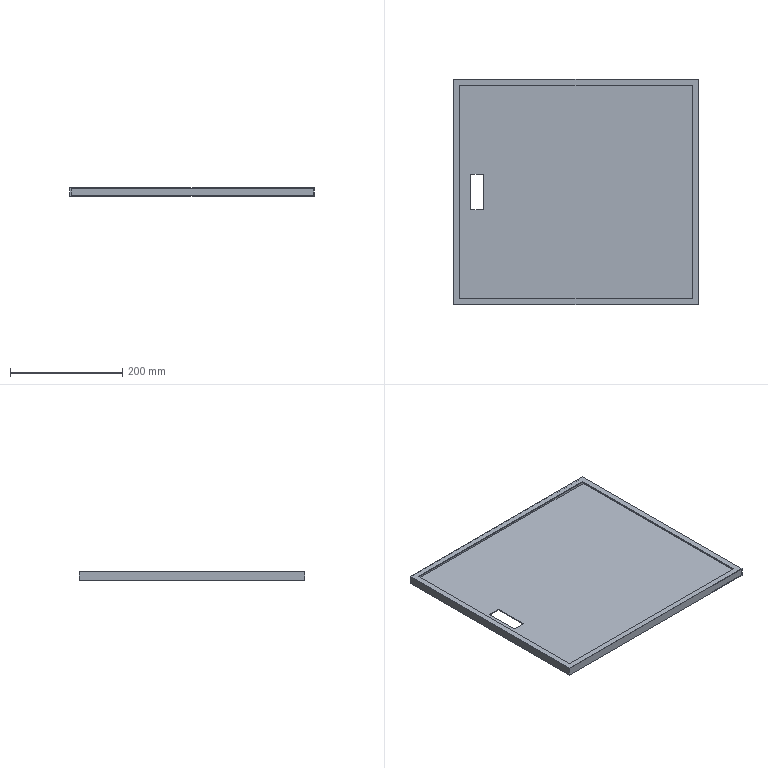Part | 1 solid | 20 faces | box 435.25 x 401 x 15 mm | volume 314971 mm3 | plane 20
STEP:
#1=CARTESIAN_POINT('',(435.25,0.,-625.));
#2=VERTEX_POINT('',#1);
#3=CARTESIAN_POINT('',(435.25,401.,-625.));
#4=VERTEX_POINT('',#3);
#5=CARTESIAN_POINT('',(435.25,0.,-625.));
#6=DIRECTION('',(0.,1.,0.));
#7=VECTOR('',#6,1000.);
#8=LINE('',#5,#7);
#9=EDGE_CURVE('',#2,#4,#8,.T.);
#10=ORIENTED_EDGE('',*,*,#9,.F.);
#11=CARTESIAN_POINT('',(435.25,0.,-640.));
#12=VERTEX_POINT('',#11);
#13=CARTESIAN_POINT('',(435.25,0.,-640.));
#14=DIRECTION('',(0.,0.,1.));
#15=VECTOR('',#14,1000.);
#16=LINE('',#13,#15);
#17=EDGE_CURVE('',#12,#2,#16,.T.);
#18=ORIENTED_EDGE('',*,*,#17,.F.);
#19=CARTESIAN_POINT('',(435.25,401.,-640.));
#20=VERTEX_POINT('',#19);
#21=CARTESIAN_POINT('',(435.25,0.,-640.));
#22=DIRECTION('',(0.,1.,0.));
#23=VECTOR('',#22,1000.);
#24=LINE('',#21,#23);
#25=EDGE_CURVE('',#12,#20,#24,.T.);
#26=ORIENTED_EDGE('',*,*,#25,.T.);
#27=CARTESIAN_POINT('',(435.25,401.,-640.));
#28=DIRECTION('',(0.,0.,1.));
#29=VECTOR('',#28,1000.);
#30=LINE('',#27,#29);
#31=EDGE_CURVE('',#20,#4,#30,.T.);
#32=ORIENTED_EDGE('',*,*,#31,.T.);
#33=EDGE_LOOP('',(#10,#18,#26,#32));
#34=FACE_OUTER_BOUND('',#33,.T.);
#35=CARTESIAN_POINT('',(435.25,0.,-640.));
#36=DIRECTION('',(1.,0.,0.));
#37=DIRECTION('',(0.,1.,0.));
#38=AXIS2_PLACEMENT_3D('',#35,#36,#37);
#39=PLANE('',#38);
#40=ADVANCED_FACE('',(#34),#39,.T.);
#41=CARTESIAN_POINT('',(0.,0.,-625.));
#42=VERTEX_POINT('',#41);
#43=CARTESIAN_POINT('',(0.,0.,-625.));
#44=DIRECTION('',(1.,0.,0.));
#45=VECTOR('',#44,1000.);
#46=LINE('',#43,#45);
#47=EDGE_CURVE('',#42,#2,#46,.T.);
#48=ORIENTED_EDGE('',*,*,#47,.F.);
#49=CARTESIAN_POINT('',(0.,0.,-640.));
#50=VERTEX_POINT('',#49);
#51=CARTESIAN_POINT('',(0.,0.,-640.));
#52=DIRECTION('',(0.,0.,1.));
#53=VECTOR('',#52,1000.);
#54=LINE('',#51,#53);
#55=EDGE_CURVE('',#50,#42,#54,.T.);
#56=ORIENTED_EDGE('',*,*,#55,.F.);
#57=CARTESIAN_POINT('',(0.,0.,-640.));
#58=DIRECTION('',(1.,0.,0.));
#59=VECTOR('',#58,1000.);
#60=LINE('',#57,#59);
#61=EDGE_CURVE('',#50,#12,#60,.T.);
#62=ORIENTED_EDGE('',*,*,#61,.T.);
#63=ORIENTED_EDGE('',*,*,#17,.T.);
#64=EDGE_LOOP('',(#48,#56,#62,#63));
#65=FACE_OUTER_BOUND('',#64,.T.);
#66=CARTESIAN_POINT('',(0.,0.,-640.));
#67=DIRECTION('',(0.,-1.,0.));
#68=DIRECTION('',(0.,0.,-1.));
#69=AXIS2_PLACEMENT_3D('',#66,#67,#68);
#70=PLANE('',#69);
#71=ADVANCED_FACE('',(#65),#70,.T.);
#72=CARTESIAN_POINT('',(0.,401.,-625.));
#73=VERTEX_POINT('',#72);
#74=CARTESIAN_POINT('',(0.,401.,-625.));
#75=DIRECTION('',(0.,-1.,0.));
#76=VECTOR('',#75,1000.);
#77=LINE('',#74,#76);
#78=EDGE_CURVE('',#73,#42,#77,.T.);
#79=ORIENTED_EDGE('',*,*,#78,.F.);
#80=CARTESIAN_POINT('',(0.,401.,-640.));
#81=VERTEX_POINT('',#80);
#82=CARTESIAN_POINT('',(0.,401.,-640.));
#83=DIRECTION('',(0.,0.,1.));
#84=VECTOR('',#83,1000.);
#85=LINE('',#82,#84);
#86=EDGE_CURVE('',#81,#73,#85,.T.);
#87=ORIENTED_EDGE('',*,*,#86,.F.);
#88=CARTESIAN_POINT('',(0.,401.,-640.));
#89=DIRECTION('',(0.,-1.,0.));
#90=VECTOR('',#89,1000.);
#91=LINE('',#88,#90);
#92=EDGE_CURVE('',#81,#50,#91,.T.);
#93=ORIENTED_EDGE('',*,*,#92,.T.);
#94=ORIENTED_EDGE('',*,*,#55,.T.);
#95=EDGE_LOOP('',(#79,#87,#93,#94));
#96=FACE_OUTER_BOUND('',#95,.T.);
#97=CARTESIAN_POINT('',(0.,401.,-640.));
#98=DIRECTION('',(-1.,0.,0.));
#99=DIRECTION('',(0.,-1.,0.));
#100=AXIS2_PLACEMENT_3D('',#97,#98,#99);
#101=PLANE('',#100);
#102=ADVANCED_FACE('',(#96),#101,.T.);
#103=CARTESIAN_POINT('',(435.25,401.,-625.));
#104=DIRECTION('',(-1.,0.,0.));
#105=VECTOR('',#104,1000.);
#106=LINE('',#103,#105);
#107=EDGE_CURVE('',#4,#73,#106,.T.);
#108=ORIENTED_EDGE('',*,*,#107,.F.);
#109=ORIENTED_EDGE('',*,*,#31,.F.);
#110=CARTESIAN_POINT('',(435.25,401.,-640.));
#111=DIRECTION('',(-1.,0.,0.));
#112=VECTOR('',#111,1000.);
#113=LINE('',#110,#112);
#114=EDGE_CURVE('',#20,#81,#113,.T.);
#115=ORIENTED_EDGE('',*,*,#114,.T.);
#116=ORIENTED_EDGE('',*,*,#86,.T.);
#117=EDGE_LOOP('',(#108,#109,#115,#116));
#118=FACE_OUTER_BOUND('',#117,.T.);
#119=CARTESIAN_POINT('',(435.25,401.,-640.));
#120=DIRECTION('',(0.,1.,0.));
#121=DIRECTION('',(0.,0.,1.));
#122=AXIS2_PLACEMENT_3D('',#119,#120,#121);
#123=PLANE('',#122);
#124=ADVANCED_FACE('',(#118),#123,.T.);
#125=CARTESIAN_POINT('',(30.,232.,-640.));
#126=VERTEX_POINT('',#125);
#127=CARTESIAN_POINT('',(53.,232.,-640.));
#128=VERTEX_POINT('',#127);
#129=CARTESIAN_POINT('',(53.,232.,-640.));
#130=DIRECTION('',(1.,0.,0.));
#131=VECTOR('',#130,1000.);
#132=LINE('',#129,#131);
#133=EDGE_CURVE('',#126,#128,#132,.T.);
#134=ORIENTED_EDGE('',*,*,#133,.F.);
#135=CARTESIAN_POINT('',(30.,169.,-640.));
#136=VERTEX_POINT('',#135);
#137=CARTESIAN_POINT('',(30.,232.,-640.));
#138=DIRECTION('',(0.,1.,0.));
#139=VECTOR('',#138,1000.);
#140=LINE('',#137,#139);
#141=EDGE_CURVE('',#136,#126,#140,.T.);
#142=ORIENTED_EDGE('',*,*,#141,.F.);
#143=CARTESIAN_POINT('',(53.,169.,-640.));
#144=VERTEX_POINT('',#143);
#145=CARTESIAN_POINT('',(53.,169.,-640.));
#146=DIRECTION('',(-1.,0.,0.));
#147=VECTOR('',#146,1000.);
#148=LINE('',#145,#147);
#149=EDGE_CURVE('',#144,#136,#148,.T.);
#150=ORIENTED_EDGE('',*,*,#149,.F.);
#151=CARTESIAN_POINT('',(53.,232.,-640.));
#152=DIRECTION('',(0.,-1.,0.));
#153=VECTOR('',#152,1000.);
#154=LINE('',#151,#153);
#155=EDGE_CURVE('',#128,#144,#154,.T.);
#156=ORIENTED_EDGE('',*,*,#155,.F.);
#157=EDGE_LOOP('',(#134,#142,#150,#156));
#158=FACE_BOUND('',#157,.T.);
#159=ORIENTED_EDGE('',*,*,#25,.F.);
#160=ORIENTED_EDGE('',*,*,#61,.F.);
#161=ORIENTED_EDGE('',*,*,#92,.F.);
#162=ORIENTED_EDGE('',*,*,#114,.F.);
#163=EDGE_LOOP('',(#159,#160,#161,#162));
#164=FACE_OUTER_BOUND('',#163,.T.);
#165=CARTESIAN_POINT('',(0.,0.,-640.));
#166=DIRECTION('',(0.,0.,1.));
#167=DIRECTION('',(1.,0.,0.));
#168=AXIS2_PLACEMENT_3D('',#165,#166,#167);
#169=PLANE('',#168);
#170=ADVANCED_FACE('',(#158,#164),#169,.F.);
#171=CARTESIAN_POINT('',(424.5,10.,-625.));
#172=VERTEX_POINT('',#171);
#173=CARTESIAN_POINT('',(10.75,10.,-625.));
#174=VERTEX_POINT('',#173);
#175=CARTESIAN_POINT('',(424.5,10.,-625.));
#176=DIRECTION('',(-1.,0.,0.));
#177=VECTOR('',#176,1000.);
#178=LINE('',#175,#177);
#179=EDGE_CURVE('',#172,#174,#178,.T.);
#180=ORIENTED_EDGE('',*,*,#179,.T.);
#181=CARTESIAN_POINT('',(10.75,391.,-625.));
#182=VERTEX_POINT('',#181);
#183=CARTESIAN_POINT('',(10.75,10.,-625.));
#184=DIRECTION('',(0.,1.,0.));
#185=VECTOR('',#184,1000.);
#186=LINE('',#183,#185);
#187=EDGE_CURVE('',#174,#182,#186,.T.);
#188=ORIENTED_EDGE('',*,*,#187,.T.);
#189=CARTESIAN_POINT('',(424.5,391.,-625.));
#190=VERTEX_POINT('',#189);
#191=CARTESIAN_POINT('',(10.75,391.,-625.));
#192=DIRECTION('',(1.,0.,0.));
#193=VECTOR('',#192,1000.);
#194=LINE('',#191,#193);
#195=EDGE_CURVE('',#182,#190,#194,.T.);
#196=ORIENTED_EDGE('',*,*,#195,.T.);
#197=CARTESIAN_POINT('',(424.5,391.,-625.));
#198=DIRECTION('',(0.,-1.,0.));
#199=VECTOR('',#198,1000.);
#200=LINE('',#197,#199);
#201=EDGE_CURVE('',#190,#172,#200,.T.);
#202=ORIENTED_EDGE('',*,*,#201,.T.);
#203=EDGE_LOOP('',(#180,#188,#196,#202));
#204=FACE_BOUND('',#203,.T.);
#205=ORIENTED_EDGE('',*,*,#9,.T.);
#206=ORIENTED_EDGE('',*,*,#107,.T.);
#207=ORIENTED_EDGE('',*,*,#78,.T.);
#208=ORIENTED_EDGE('',*,*,#47,.T.);
#209=EDGE_LOOP('',(#205,#206,#207,#208));
#210=FACE_OUTER_BOUND('',#209,.T.);
#211=CARTESIAN_POINT('',(0.,0.,-625.));
#212=DIRECTION('',(0.,0.,1.));
#213=DIRECTION('',(1.,0.,0.));
#214=AXIS2_PLACEMENT_3D('',#211,#212,#213);
#215=PLANE('',#214);
#216=ADVANCED_FACE('',(#204,#210),#215,.T.);
#217=CARTESIAN_POINT('',(424.5,10.,-626.5));
#218=VERTEX_POINT('',#217);
#219=CARTESIAN_POINT('',(10.75,10.,-626.5));
#220=VERTEX_POINT('',#219);
#221=CARTESIAN_POINT('',(424.5,10.,-626.5));
#222=DIRECTION('',(-1.,0.,0.));
#223=VECTOR('',#222,1000.);
#224=LINE('',#221,#223);
#225=EDGE_CURVE('',#218,#220,#224,.T.);
#226=ORIENTED_EDGE('',*,*,#225,.T.);
#227=CARTESIAN_POINT('',(10.75,10.,-625.));
#228=DIRECTION('',(0.,0.,-1.));
#229=VECTOR('',#228,1000.);
#230=LINE('',#227,#229);
#231=EDGE_CURVE('',#174,#220,#230,.T.);
#232=ORIENTED_EDGE('',*,*,#231,.F.);
#233=ORIENTED_EDGE('',*,*,#179,.F.);
#234=CARTESIAN_POINT('',(424.5,10.,-625.));
#235=DIRECTION('',(0.,0.,-1.));
#236=VECTOR('',#235,1000.);
#237=LINE('',#234,#236);
#238=EDGE_CURVE('',#172,#218,#237,.T.);
#239=ORIENTED_EDGE('',*,*,#238,.T.);
#240=EDGE_LOOP('',(#226,#232,#233,#239));
#241=FACE_OUTER_BOUND('',#240,.T.);
#242=CARTESIAN_POINT('',(424.5,10.,-625.));
#243=DIRECTION('',(0.,-1.,0.));
#244=DIRECTION('',(1.,0.,0.));
#245=AXIS2_PLACEMENT_3D('',#242,#243,#244);
#246=PLANE('',#245);
#247=ADVANCED_FACE('',(#241),#246,.F.);
#248=CARTESIAN_POINT('',(424.5,391.,-626.5));
#249=VERTEX_POINT('',#248);
#250=CARTESIAN_POINT('',(424.5,391.,-626.5));
#251=DIRECTION('',(0.,-1.,0.));
#252=VECTOR('',#251,1000.);
#253=LINE('',#250,#252);
#254=EDGE_CURVE('',#249,#218,#253,.T.);
#255=ORIENTED_EDGE('',*,*,#254,.T.);
#256=ORIENTED_EDGE('',*,*,#238,.F.);
#257=ORIENTED_EDGE('',*,*,#201,.F.);
#258=CARTESIAN_POINT('',(424.5,391.,-625.));
#259=DIRECTION('',(0.,0.,-1.));
#260=VECTOR('',#259,1000.);
#261=LINE('',#258,#260);
#262=EDGE_CURVE('',#190,#249,#261,.T.);
#263=ORIENTED_EDGE('',*,*,#262,.T.);
#264=EDGE_LOOP('',(#255,#256,#257,#263));
#265=FACE_OUTER_BOUND('',#264,.T.);
#266=CARTESIAN_POINT('',(424.5,391.,-625.));
#267=DIRECTION('',(1.,0.,0.));
#268=DIRECTION('',(0.,1.,0.));
#269=AXIS2_PLACEMENT_3D('',#266,#267,#268);
#270=PLANE('',#269);
#271=ADVANCED_FACE('',(#265),#270,.F.);
#272=CARTESIAN_POINT('',(10.75,391.,-626.5));
#273=VERTEX_POINT('',#272);
#274=CARTESIAN_POINT('',(10.75,391.,-626.5));
#275=DIRECTION('',(1.,0.,0.));
#276=VECTOR('',#275,1000.);
#277=LINE('',#274,#276);
#278=EDGE_CURVE('',#273,#249,#277,.T.);
#279=ORIENTED_EDGE('',*,*,#278,.T.);
#280=ORIENTED_EDGE('',*,*,#262,.F.);
#281=ORIENTED_EDGE('',*,*,#195,.F.);
#282=CARTESIAN_POINT('',(10.75,391.,-625.));
#283=DIRECTION('',(0.,0.,-1.));
#284=VECTOR('',#283,1000.);
#285=LINE('',#282,#284);
#286=EDGE_CURVE('',#182,#273,#285,.T.);
#287=ORIENTED_EDGE('',*,*,#286,.T.);
#288=EDGE_LOOP('',(#279,#280,#281,#287));
#289=FACE_OUTER_BOUND('',#288,.T.);
#290=CARTESIAN_POINT('',(10.75,391.,-625.));
#291=DIRECTION('',(0.,1.,0.));
#292=DIRECTION('',(-1.,0.,0.));
#293=AXIS2_PLACEMENT_3D('',#290,#291,#292);
#294=PLANE('',#293);
#295=ADVANCED_FACE('',(#289),#294,.F.);
#296=CARTESIAN_POINT('',(10.75,10.,-626.5));
#297=DIRECTION('',(0.,1.,0.));
#298=VECTOR('',#297,1000.);
#299=LINE('',#296,#298);
#300=EDGE_CURVE('',#220,#273,#299,.T.);
#301=ORIENTED_EDGE('',*,*,#300,.T.);
#302=ORIENTED_EDGE('',*,*,#286,.F.);
#303=ORIENTED_EDGE('',*,*,#187,.F.);
#304=ORIENTED_EDGE('',*,*,#231,.T.);
#305=EDGE_LOOP('',(#301,#302,#303,#304));
#306=FACE_OUTER_BOUND('',#305,.T.);
#307=CARTESIAN_POINT('',(10.75,10.,-625.));
#308=DIRECTION('',(-1.,0.,0.));
#309=DIRECTION('',(0.,-1.,0.));
#310=AXIS2_PLACEMENT_3D('',#307,#308,#309);
#311=PLANE('',#310);
#312=ADVANCED_FACE('',(#306),#311,.F.);
#313=CARTESIAN_POINT('',(2.25,1.5,-626.5));
#314=VERTEX_POINT('',#313);
#315=CARTESIAN_POINT('',(2.25,399.5,-626.5));
#316=VERTEX_POINT('',#315);
#317=CARTESIAN_POINT('',(2.25,1.5,-626.5));
#318=DIRECTION('',(0.,1.,0.));
#319=VECTOR('',#318,1000.);
#320=LINE('',#317,#319);
#321=EDGE_CURVE('',#314,#316,#320,.T.);
#322=ORIENTED_EDGE('',*,*,#321,.T.);
#323=CARTESIAN_POINT('',(434.5,399.5,-626.5));
#324=VERTEX_POINT('',#323);
#325=CARTESIAN_POINT('',(434.5,399.5,-626.5));
#326=DIRECTION('',(-1.,0.,0.));
#327=VECTOR('',#326,1000.);
#328=LINE('',#325,#327);
#329=EDGE_CURVE('',#324,#316,#328,.T.);
#330=ORIENTED_EDGE('',*,*,#329,.F.);
#331=CARTESIAN_POINT('',(434.5,1.5,-626.5));
#332=VERTEX_POINT('',#331);
#333=CARTESIAN_POINT('',(434.5,1.5,-626.5));
#334=DIRECTION('',(0.,1.,0.));
#335=VECTOR('',#334,1000.);
#336=LINE('',#333,#335);
#337=EDGE_CURVE('',#332,#324,#336,.T.);
#338=ORIENTED_EDGE('',*,*,#337,.F.);
#339=CARTESIAN_POINT('',(434.5,1.5,-626.5));
#340=DIRECTION('',(-1.,0.,0.));
#341=VECTOR('',#340,1000.);
#342=LINE('',#339,#341);
#343=EDGE_CURVE('',#332,#314,#342,.T.);
#344=ORIENTED_EDGE('',*,*,#343,.T.);
#345=EDGE_LOOP('',(#322,#330,#338,#344));
#346=FACE_OUTER_BOUND('',#345,.T.);
#347=ORIENTED_EDGE('',*,*,#225,.F.);
#348=ORIENTED_EDGE('',*,*,#254,.F.);
#349=ORIENTED_EDGE('',*,*,#278,.F.);
#350=ORIENTED_EDGE('',*,*,#300,.F.);
#351=EDGE_LOOP('',(#347,#348,#349,#350));
#352=FACE_BOUND('',#351,.T.);
#353=CARTESIAN_POINT('',(434.5,1.5,-626.5));
#354=DIRECTION('',(0.,0.,1.));
#355=DIRECTION('',(0.,-1.,0.));
#356=AXIS2_PLACEMENT_3D('',#353,#354,#355);
#357=PLANE('',#356);
#358=ADVANCED_FACE('',(#346,#352),#357,.F.);
#359=CARTESIAN_POINT('',(2.25,1.5,-638.5));
#360=VERTEX_POINT('',#359);
#361=CARTESIAN_POINT('',(2.25,1.5,-638.5));
#362=DIRECTION('',(0.,0.,1.));
#363=VECTOR('',#362,1000.);
#364=LINE('',#361,#363);
#365=EDGE_CURVE('',#360,#314,#364,.T.);
#366=ORIENTED_EDGE('',*,*,#365,.T.);
#367=ORIENTED_EDGE('',*,*,#343,.F.);
#368=CARTESIAN_POINT('',(434.5,1.5,-638.5));
#369=VERTEX_POINT('',#368);
#370=CARTESIAN_POINT('',(434.5,1.5,-638.5));
#371=DIRECTION('',(0.,0.,1.));
#372=VECTOR('',#371,1000.);
#373=LINE('',#370,#372);
#374=EDGE_CURVE('',#369,#332,#373,.T.);
#375=ORIENTED_EDGE('',*,*,#374,.F.);
#376=CARTESIAN_POINT('',(434.5,1.5,-638.5));
#377=DIRECTION('',(-1.,0.,0.));
#378=VECTOR('',#377,1000.);
#379=LINE('',#376,#378);
#380=EDGE_CURVE('',#369,#360,#379,.T.);
#381=ORIENTED_EDGE('',*,*,#380,.T.);
#382=EDGE_LOOP('',(#366,#367,#375,#381));
#383=FACE_OUTER_BOUND('',#382,.T.);
#384=CARTESIAN_POINT('',(434.5,1.5,-638.5));
#385=DIRECTION('',(0.,-1.,0.));
#386=DIRECTION('',(0.,0.,-1.));
#387=AXIS2_PLACEMENT_3D('',#384,#385,#386);
#388=PLANE('',#387);
#389=ADVANCED_FACE('',(#383),#388,.F.);
#390=CARTESIAN_POINT('',(53.,169.,-638.5));
#391=VERTEX_POINT('',#390);
#392=CARTESIAN_POINT('',(30.,169.,-638.5));
#393=VERTEX_POINT('',#392);
#394=CARTESIAN_POINT('',(434.5,169.,-638.5));
#395=DIRECTION('',(-1.,0.,0.));
#396=VECTOR('',#395,1000.);
#397=LINE('',#394,#396);
#398=EDGE_CURVE('',#391,#393,#397,.T.);
#399=ORIENTED_EDGE('',*,*,#398,.T.);
#400=CARTESIAN_POINT('',(30.,232.,-638.5));
#401=VERTEX_POINT('',#400);
#402=CARTESIAN_POINT('',(30.,399.5,-638.5));
#403=DIRECTION('',(0.,1.,0.));
#404=VECTOR('',#403,1000.);
#405=LINE('',#402,#404);
#406=EDGE_CURVE('',#393,#401,#405,.T.);
#407=ORIENTED_EDGE('',*,*,#406,.T.);
#408=CARTESIAN_POINT('',(53.,232.,-638.5));
#409=VERTEX_POINT('',#408);
#410=CARTESIAN_POINT('',(434.5,232.,-638.5));
#411=DIRECTION('',(1.,0.,0.));
#412=VECTOR('',#411,1000.);
#413=LINE('',#410,#412);
#414=EDGE_CURVE('',#401,#409,#413,.T.);
#415=ORIENTED_EDGE('',*,*,#414,.T.);
#416=CARTESIAN_POINT('',(53.,399.5,-638.5));
#417=DIRECTION('',(0.,-1.,0.));
#418=VECTOR('',#417,1000.);
#419=LINE('',#416,#418);
#420=EDGE_CURVE('',#409,#391,#419,.T.);
#421=ORIENTED_EDGE('',*,*,#420,.T.);
#422=EDGE_LOOP('',(#399,#407,#415,#421));
#423=FACE_BOUND('',#422,.T.);
#424=CARTESIAN_POINT('',(2.25,399.5,-638.5));
#425=VERTEX_POINT('',#424);
#426=CARTESIAN_POINT('',(2.25,399.5,-638.5));
#427=DIRECTION('',(0.,-1.,0.));
#428=VECTOR('',#427,1000.);
#429=LINE('',#426,#428);
#430=EDGE_CURVE('',#425,#360,#429,.T.);
#431=ORIENTED_EDGE('',*,*,#430,.T.);
#432=ORIENTED_EDGE('',*,*,#380,.F.);
#433=CARTESIAN_POINT('',(434.5,399.5,-638.5));
#434=VERTEX_POINT('',#433);
#435=CARTESIAN_POINT('',(434.5,399.5,-638.5));
#436=DIRECTION('',(0.,-1.,0.));
#437=VECTOR('',#436,1000.);
#438=LINE('',#435,#437);
#439=EDGE_CURVE('',#434,#369,#438,.T.);
#440=ORIENTED_EDGE('',*,*,#439,.F.);
#441=CARTESIAN_POINT('',(434.5,399.5,-638.5));
#442=DIRECTION('',(-1.,0.,0.));
#443=VECTOR('',#442,1000.);
#444=LINE('',#441,#443);
#445=EDGE_CURVE('',#434,#425,#444,.T.);
#446=ORIENTED_EDGE('',*,*,#445,.T.);
#447=EDGE_LOOP('',(#431,#432,#440,#446));
#448=FACE_OUTER_BOUND('',#447,.T.);
#449=CARTESIAN_POINT('',(434.5,399.5,-638.5));
#450=DIRECTION('',(0.,0.,-1.));
#451=DIRECTION('',(-1.,0.,0.));
#452=AXIS2_PLACEMENT_3D('',#449,#450,#451);
#453=PLANE('',#452);
#454=ADVANCED_FACE('',(#423,#448),#453,.F.);
#455=CARTESIAN_POINT('',(2.25,399.5,-626.5));
#456=DIRECTION('',(0.,0.,-1.));
#457=VECTOR('',#456,1000.);
#458=LINE('',#455,#457);
#459=EDGE_CURVE('',#316,#425,#458,.T.);
#460=ORIENTED_EDGE('',*,*,#459,.T.);
#461=ORIENTED_EDGE('',*,*,#445,.F.);
#462=CARTESIAN_POINT('',(434.5,399.5,-626.5));
#463=DIRECTION('',(0.,0.,-1.));
#464=VECTOR('',#463,1000.);
#465=LINE('',#462,#464);
#466=EDGE_CURVE('',#324,#434,#465,.T.);
#467=ORIENTED_EDGE('',*,*,#466,.F.);
#468=ORIENTED_EDGE('',*,*,#329,.T.);
#469=EDGE_LOOP('',(#460,#461,#467,#468));
#470=FACE_OUTER_BOUND('',#469,.T.);
#471=CARTESIAN_POINT('',(434.5,399.5,-626.5));
#472=DIRECTION('',(0.,1.,0.));
#473=DIRECTION('',(0.,0.,1.));
#474=AXIS2_PLACEMENT_3D('',#471,#472,#473);
#475=PLANE('',#474);
#476=ADVANCED_FACE('',(#470),#475,.F.);
#477=ORIENTED_EDGE('',*,*,#337,.T.);
#478=ORIENTED_EDGE('',*,*,#466,.T.);
#479=ORIENTED_EDGE('',*,*,#439,.T.);
#480=ORIENTED_EDGE('',*,*,#374,.T.);
#481=EDGE_LOOP('',(#477,#478,#479,#480));
#482=FACE_OUTER_BOUND('',#481,.T.);
#483=CARTESIAN_POINT('',(434.5,0.,0.));
#484=DIRECTION('',(-1.,0.,0.));
#485=DIRECTION('',(0.,0.,1.));
#486=AXIS2_PLACEMENT_3D('',#483,#484,#485);
#487=PLANE('',#486);
#488=ADVANCED_FACE('',(#482),#487,.T.);
#489=ORIENTED_EDGE('',*,*,#321,.F.);
#490=ORIENTED_EDGE('',*,*,#365,.F.);
#491=ORIENTED_EDGE('',*,*,#430,.F.);
#492=ORIENTED_EDGE('',*,*,#459,.F.);
#493=EDGE_LOOP('',(#489,#490,#491,#492));
#494=FACE_OUTER_BOUND('',#493,.T.);
#495=CARTESIAN_POINT('',(2.25,0.,0.));
#496=DIRECTION('',(-1.,0.,0.));
#497=DIRECTION('',(0.,0.,1.));
#498=AXIS2_PLACEMENT_3D('',#495,#496,#497);
#499=PLANE('',#498);
#500=ADVANCED_FACE('',(#494),#499,.F.);
#501=CARTESIAN_POINT('',(30.,169.,-630.));
#502=DIRECTION('',(0.,0.,-1.));
#503=VECTOR('',#502,1000.);
#504=LINE('',#501,#503);
#505=EDGE_CURVE('',#393,#136,#504,.T.);
#506=ORIENTED_EDGE('',*,*,#505,.T.);
#507=ORIENTED_EDGE('',*,*,#141,.T.);
#508=CARTESIAN_POINT('',(30.,232.,-630.));
#509=DIRECTION('',(0.,0.,-1.));
#510=VECTOR('',#509,1000.);
#511=LINE('',#508,#510);
#512=EDGE_CURVE('',#401,#126,#511,.T.);
#513=ORIENTED_EDGE('',*,*,#512,.F.);
#514=ORIENTED_EDGE('',*,*,#406,.F.);
#515=EDGE_LOOP('',(#506,#507,#513,#514));
#516=FACE_OUTER_BOUND('',#515,.T.);
#517=CARTESIAN_POINT('',(30.,232.,-630.));
#518=DIRECTION('',(-1.,0.,0.));
#519=DIRECTION('',(0.,-1.,0.));
#520=AXIS2_PLACEMENT_3D('',#517,#518,#519);
#521=PLANE('',#520);
#522=ADVANCED_FACE('',(#516),#521,.F.);
#523=CARTESIAN_POINT('',(53.,169.,-630.));
#524=DIRECTION('',(0.,0.,-1.));
#525=VECTOR('',#524,1000.);
#526=LINE('',#523,#525);
#527=EDGE_CURVE('',#391,#144,#526,.T.);
#528=ORIENTED_EDGE('',*,*,#527,.T.);
#529=ORIENTED_EDGE('',*,*,#149,.T.);
#530=ORIENTED_EDGE('',*,*,#505,.F.);
#531=ORIENTED_EDGE('',*,*,#398,.F.);
#532=EDGE_LOOP('',(#528,#529,#530,#531));
#533=FACE_OUTER_BOUND('',#532,.T.);
#534=CARTESIAN_POINT('',(53.,169.,-630.));
#535=DIRECTION('',(0.,-1.,0.));
#536=DIRECTION('',(1.,0.,0.));
#537=AXIS2_PLACEMENT_3D('',#534,#535,#536);
#538=PLANE('',#537);
#539=ADVANCED_FACE('',(#533),#538,.F.);
#540=CARTESIAN_POINT('',(53.,232.,-630.));
#541=DIRECTION('',(0.,0.,-1.));
#542=VECTOR('',#541,1000.);
#543=LINE('',#540,#542);
#544=EDGE_CURVE('',#409,#128,#543,.T.);
#545=ORIENTED_EDGE('',*,*,#544,.T.);
#546=ORIENTED_EDGE('',*,*,#155,.T.);
#547=ORIENTED_EDGE('',*,*,#527,.F.);
#548=ORIENTED_EDGE('',*,*,#420,.F.);
#549=EDGE_LOOP('',(#545,#546,#547,#548));
#550=FACE_OUTER_BOUND('',#549,.T.);
#551=CARTESIAN_POINT('',(53.,232.,-630.));
#552=DIRECTION('',(1.,0.,0.));
#553=DIRECTION('',(0.,1.,0.));
#554=AXIS2_PLACEMENT_3D('',#551,#552,#553);
#555=PLANE('',#554);
#556=ADVANCED_FACE('',(#550),#555,.F.);
#557=ORIENTED_EDGE('',*,*,#512,.T.);
#558=ORIENTED_EDGE('',*,*,#133,.T.);
#559=ORIENTED_EDGE('',*,*,#544,.F.);
#560=ORIENTED_EDGE('',*,*,#414,.F.);
#561=EDGE_LOOP('',(#557,#558,#559,#560));
#562=FACE_OUTER_BOUND('',#561,.T.);
#563=CARTESIAN_POINT('',(53.,232.,-630.));
#564=DIRECTION('',(0.,1.,0.));
#565=DIRECTION('',(-1.,0.,0.));
#566=AXIS2_PLACEMENT_3D('',#563,#564,#565);
#567=PLANE('',#566);
#568=ADVANCED_FACE('',(#562),#567,.F.);
#569=CLOSED_SHELL('',(#40,#71,#102,#124,#170,#216,#247,#271,#295,#312,#358,#389,#454,#476,#488,#500,#522,#539,#556,#568));
#570=MANIFOLD_SOLID_BREP('',#569);
#571=CARTESIAN_POINT('',(0.,0.,0.));
#572=DIRECTION('',(0.,0.,1.));
#573=DIRECTION('',(1.,0.,0.));
#574=AXIS2_PLACEMENT_3D('',#571,#572,#573);
#575=(LENGTH_UNIT()NAMED_UNIT(*)SI_UNIT(.MILLI.,.METRE.));
#576=UNCERTAINTY_MEASURE_WITH_UNIT(LENGTH_MEASURE(0.00001),#575,'','');
#577=(NAMED_UNIT(*)PLANE_ANGLE_UNIT()SI_UNIT($,.RADIAN.));
#578=(NAMED_UNIT(*)SI_UNIT($,.STERADIAN.)SOLID_ANGLE_UNIT());
#579=(GEOMETRIC_REPRESENTATION_CONTEXT(3)GLOBAL_UNCERTAINTY_ASSIGNED_CONTEXT((#576))GLOBAL_UNIT_ASSIGNED_CONTEXT((#575,#577,#578))REPRESENTATION_CONTEXT('',''));
#580=ADVANCED_BREP_SHAPE_REPRESENTATION('',(#570,#574),#579);